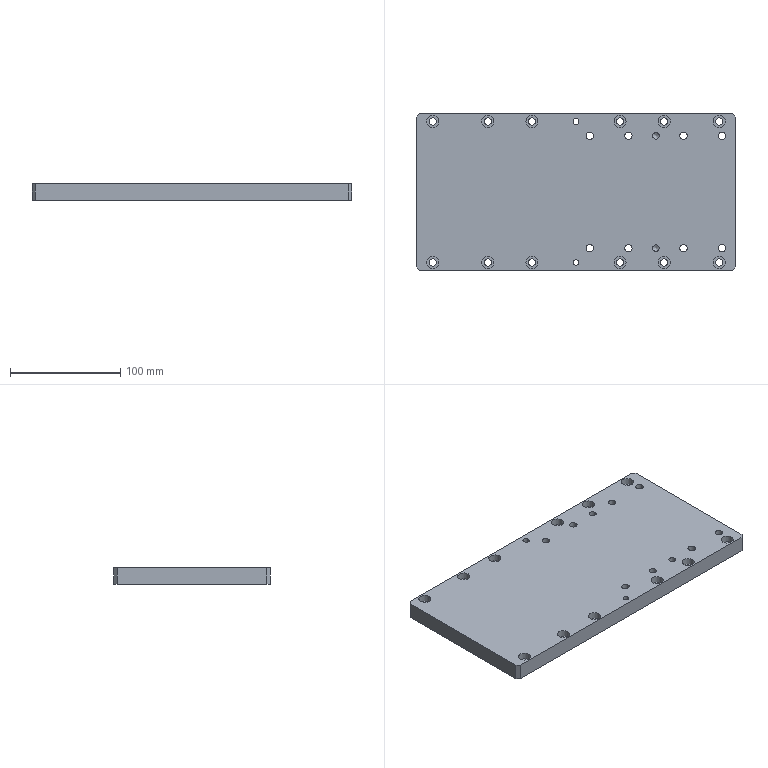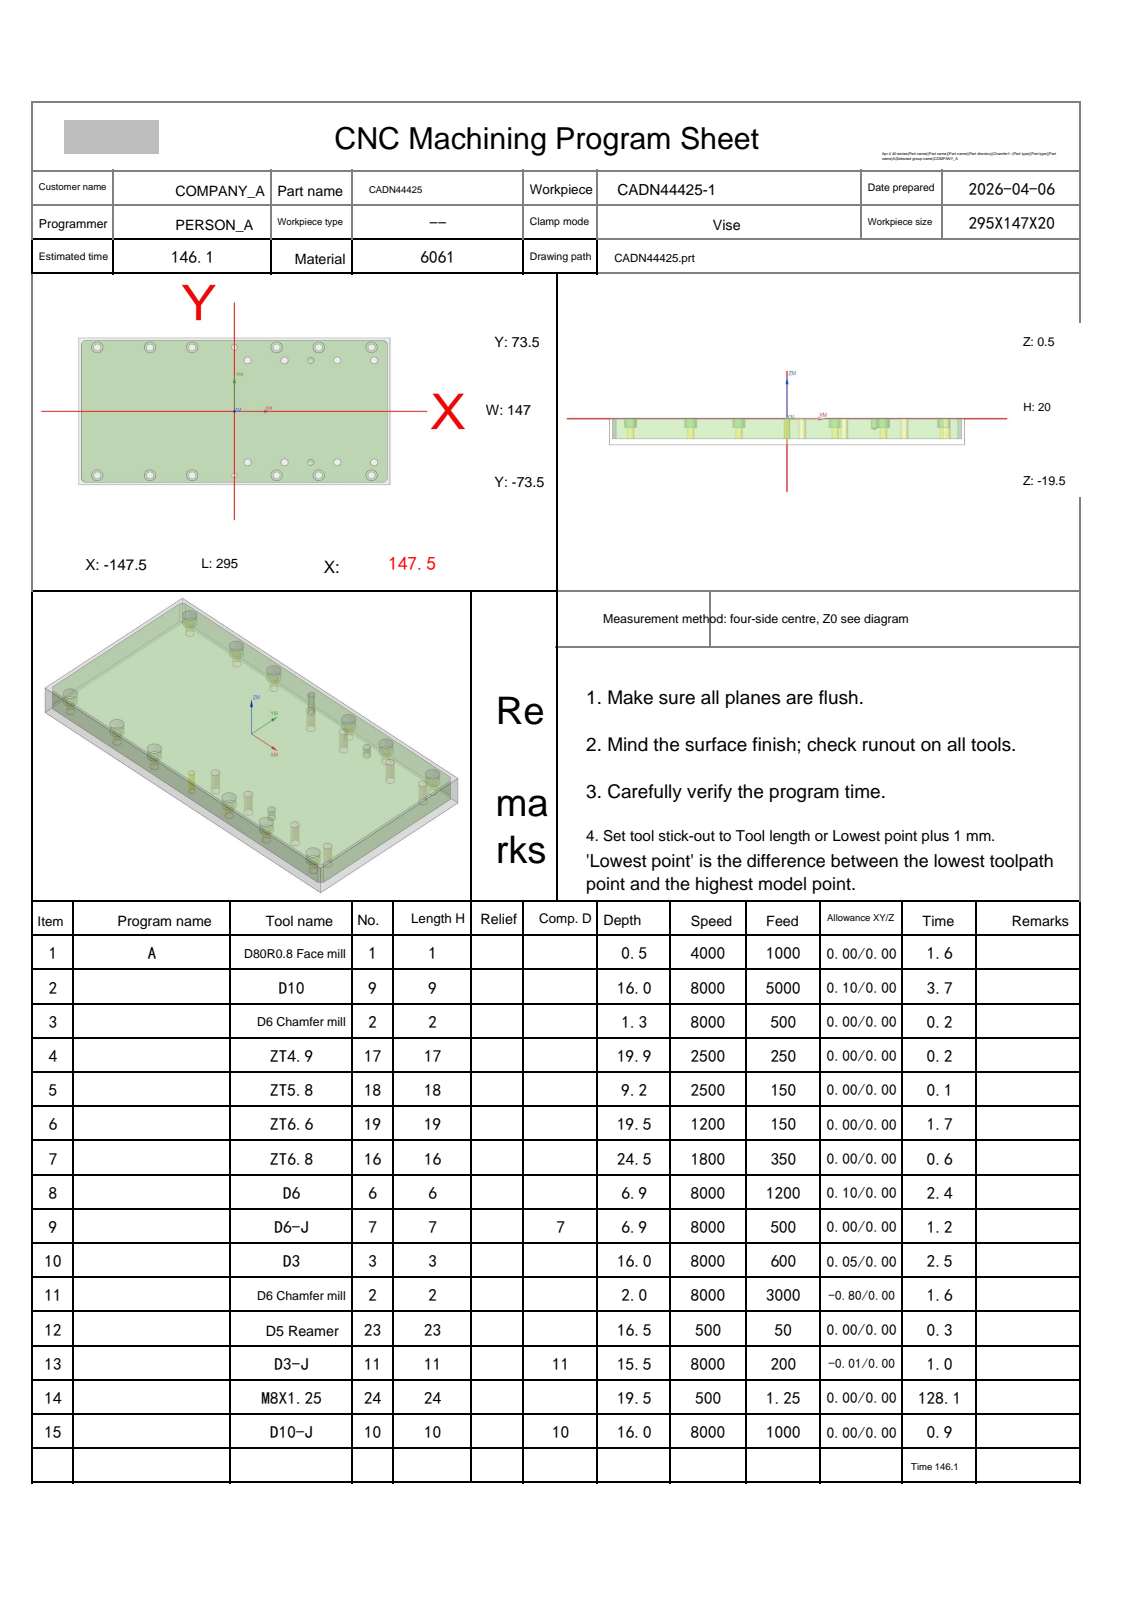NC program | NX | posted by the shop | part box 290 x 142 x 15 mm
Lines 1 to 1801 of 2582, first 1324 of 1799 lines:
%
O0001
(Machine time: 270.74 MIN)
(===Total Tool:14===)
(T1=D80R0.8 Face mill D=80.  R=0.8  D-  H01 Z=0.    )
(T9=D10     D=10.  R=0.   D-  H09 Z=-15.5 )
(T2=D6 Chamfer mill   D=6.   R=0.   D-  H02 Z=-1.5  )
(T17=ZT4.9  D=4.9  DR_a=120 D-  H17 Z=-19.41)
(T18=ZT5.8  D=5.8  DR_a=118 D-  H18 Z=-8.7  )
(T19=ZT6.6  D=6.6  DR_a=118 D-  H19 Z=-18.98)
(T16=ZT6.8  D=6.8  DR_a=118 D-  H16 Z=-24.04)
(T6=D6      D=6.   R=0.   D-  H06 Z=-6.4  )
(T7=D6-J    D=6.   R=0.   D7  H07 Z=-6.4  )
(T3=D3      D=3.   R=0.   D-  H03 Z=-15.5 )
(T23=D5 Reamer   D=5.   DR_a=180 D-  H23 Z=-16.  )
(T11=D3-J   D=3.   R=0.   D11 H11 Z=-15.  )
(T24=M8X1.25 D=6.8  DR_a=180 D-  H24 Z=-19.  )
(T10=D10-J  D=10.  R=0.   D10 H10 Z=-15.5 )
G80 G90 G17 G49 G40
G91 G28 Z0
M01
N1 T01 M06
(D80R0.8 Face mill  D=80. R=0.8 H=01 ce=0.00 di=0.00)
G00 G90 G54 X-190. Y66.6 M03 S4000
G43 H01 Z20.
M08
Z2.
G01 Z0.0 F1000.
X-185.
X185.
Y22.2
X-185.
Y-22.2
X185.
Y-66.6
X-185.
X-190.
Z2.
G00 Z20.
G91 G28 Z0.0
M05
M09
G91 G28 Z0.0
M01
N2 T09 M06
(D10  D=10. R=0. H=09 ce=0.10 di=0.00)
G00 G90 G54 X0.0 Y76.1 M03 S8000
G43 H09 Z20.
M08
Z.5
G01 X142. Z.372 F5000.
G02 X145.606 Y74.606 Z.369 I0.0 J-5.1
G01 X148.606 Y71.606 Z.365
G02 X150.1 Y68. Z.361 I-3.606 J-3.606
G01 Y-68. Z.239
G02 X148.606 Y-71.606 Z.235 I-5.1 J0.0
G01 X145.606 Y-74.606 Z.231
G02 X142. Y-76.1 Z.228 I-3.606 J3.606
G01 X-142. Z-.028
G02 X-145.606 Y-74.606 Z-.031 I0.0 J5.1
G01 X-148.606 Y-71.606 Z-.035
G02 X-150.1 Y-68. Z-.039 I3.606 J3.606
G01 Y68. Z-.161
G02 X-148.606 Y71.606 Z-.165 I5.1 J0.0
G01 X-145.606 Y74.606 Z-.169
G02 X-142. Y76.1 Z-.172 I3.606 J-3.606
G01 X142. Z-.428
G02 X145.606 Y74.606 Z-.431 I0.0 J-5.1
G01 X148.606 Y71.606 Z-.435
G02 X150.1 Y68. Z-.439 I-3.606 J-3.606
G01 Y-68. Z-.561
G02 X148.606 Y-71.606 Z-.565 I-5.1 J0.0
G01 X145.606 Y-74.606 Z-.569
G02 X142. Y-76.1 Z-.572 I-3.606 J3.606
G01 X-142. Z-.828
G02 X-145.606 Y-74.606 Z-.831 I0.0 J5.1
G01 X-148.606 Y-71.606 Z-.835
G02 X-150.1 Y-68. Z-.839 I3.606 J3.606
G01 Y68. Z-.961
G02 X-148.606 Y71.606 Z-.965 I5.1 J0.0
G01 X-145.606 Y74.606 Z-.969
G02 X-142. Y76.1 Z-.972 I3.606 J-3.606
G01 X142. Z-1.228
G02 X145.606 Y74.606 Z-1.231 I0.0 J-5.1
G01 X148.606 Y71.606 Z-1.235
G02 X150.1 Y68. Z-1.239 I-3.606 J-3.606
G01 Y-68. Z-1.361
G02 X148.606 Y-71.606 Z-1.365 I-5.1 J0.0
G01 X145.606 Y-74.606 Z-1.369
G02 X142. Y-76.1 Z-1.372 I-3.606 J3.606
G01 X-142. Z-1.628
G02 X-145.606 Y-74.606 Z-1.631 I0.0 J5.1
G01 X-148.606 Y-71.606 Z-1.635
G02 X-150.1 Y-68. Z-1.639 I3.606 J3.606
G01 Y68. Z-1.761
G02 X-148.606 Y71.606 Z-1.765 I5.1 J0.0
G01 X-145.606 Y74.606 Z-1.769
G02 X-142. Y76.1 Z-1.772 I3.606 J-3.606
G01 X142. Z-2.028
G02 X145.606 Y74.606 Z-2.031 I0.0 J-5.1
G01 X148.606 Y71.606 Z-2.035
G02 X150.1 Y68. Z-2.039 I-3.606 J-3.606
G01 Y-68. Z-2.161
G02 X148.606 Y-71.606 Z-2.165 I-5.1 J0.0
G01 X145.606 Y-74.606 Z-2.169
G02 X142. Y-76.1 Z-2.172 I-3.606 J3.606
G01 X-142. Z-2.428
G02 X-145.606 Y-74.606 Z-2.431 I0.0 J5.1
G01 X-148.606 Y-71.606 Z-2.435
G02 X-150.1 Y-68. Z-2.439 I3.606 J3.606
G01 Y68. Z-2.561
G02 X-148.606 Y71.606 Z-2.565 I5.1 J0.0
G01 X-145.606 Y74.606 Z-2.569
G02 X-142. Y76.1 Z-2.572 I3.606 J-3.606
G01 X142. Z-2.828
G02 X145.606 Y74.606 Z-2.831 I0.0 J-5.1
G01 X148.606 Y71.606 Z-2.835
G02 X150.1 Y68. Z-2.839 I-3.606 J-3.606
G01 Y-68. Z-2.961
G02 X148.606 Y-71.606 Z-2.965 I-5.1 J0.0
G01 X145.606 Y-74.606 Z-2.969
G02 X142. Y-76.1 Z-2.972 I-3.606 J3.606
G01 X-142. Z-3.228
G02 X-145.606 Y-74.606 Z-3.231 I0.0 J5.1
G01 X-148.606 Y-71.606 Z-3.235
G02 X-150.1 Y-68. Z-3.239 I3.606 J3.606
G01 Y68. Z-3.361
G02 X-148.606 Y71.606 Z-3.365 I5.1 J0.0
G01 X-145.606 Y74.606 Z-3.369
G02 X-142. Y76.1 Z-3.372 I3.606 J-3.606
G01 X142. Z-3.628
G02 X145.606 Y74.606 Z-3.631 I0.0 J-5.1
G01 X148.606 Y71.606 Z-3.635
G02 X150.1 Y68. Z-3.639 I-3.606 J-3.606
G01 Y-68. Z-3.761
G02 X148.606 Y-71.606 Z-3.765 I-5.1 J0.0
G01 X145.606 Y-74.606 Z-3.769
G02 X142. Y-76.1 Z-3.772 I-3.606 J3.606
G01 X-142. Z-4.028
G02 X-145.606 Y-74.606 Z-4.031 I0.0 J5.1
G01 X-148.606 Y-71.606 Z-4.035
G02 X-150.1 Y-68. Z-4.039 I3.606 J3.606
G01 Y68. Z-4.161
G02 X-148.606 Y71.606 Z-4.165 I5.1 J0.0
G01 X-145.606 Y74.606 Z-4.169
G02 X-142. Y76.1 Z-4.172 I3.606 J-3.606
G01 X142. Z-4.428
G02 X145.606 Y74.606 Z-4.431 I0.0 J-5.1
G01 X148.606 Y71.606 Z-4.435
G02 X150.1 Y68. Z-4.439 I-3.606 J-3.606
G01 Y-68. Z-4.561
G02 X148.606 Y-71.606 Z-4.565 I-5.1 J0.0
G01 X145.606 Y-74.606 Z-4.569
G02 X142. Y-76.1 Z-4.572 I-3.606 J3.606
G01 X-142. Z-4.828
G02 X-145.606 Y-74.606 Z-4.831 I0.0 J5.1
G01 X-148.606 Y-71.606 Z-4.835
G02 X-150.1 Y-68. Z-4.839 I3.606 J3.606
G01 Y68. Z-4.961
G02 X-148.606 Y71.606 Z-4.965 I5.1 J0.0
G01 X-145.606 Y74.606 Z-4.969
G02 X-142. Y76.1 Z-4.972 I3.606 J-3.606
G01 X142. Z-5.228
G02 X145.606 Y74.606 Z-5.231 I0.0 J-5.1
G01 X148.606 Y71.606 Z-5.235
G02 X150.1 Y68. Z-5.239 I-3.606 J-3.606
G01 Y-68. Z-5.361
G02 X148.606 Y-71.606 Z-5.365 I-5.1 J0.0
G01 X145.606 Y-74.606 Z-5.369
G02 X142. Y-76.1 Z-5.372 I-3.606 J3.606
G01 X-142. Z-5.628
G02 X-145.606 Y-74.606 Z-5.631 I0.0 J5.1
G01 X-148.606 Y-71.606 Z-5.635
G02 X-150.1 Y-68. Z-5.639 I3.606 J3.606
G01 Y68. Z-5.761
G02 X-148.606 Y71.606 Z-5.765 I5.1 J0.0
G01 X-145.606 Y74.606 Z-5.769
G02 X-142. Y76.1 Z-5.772 I3.606 J-3.606
G01 X142. Z-6.028
G02 X145.606 Y74.606 Z-6.031 I0.0 J-5.1
G01 X148.606 Y71.606 Z-6.035
G02 X150.1 Y68. Z-6.039 I-3.606 J-3.606
G01 Y-68. Z-6.161
G02 X148.606 Y-71.606 Z-6.165 I-5.1 J0.0
G01 X145.606 Y-74.606 Z-6.169
G02 X142. Y-76.1 Z-6.172 I-3.606 J3.606
G01 X-142. Z-6.428
G02 X-145.606 Y-74.606 Z-6.431 I0.0 J5.1
G01 X-148.606 Y-71.606 Z-6.435
G02 X-150.1 Y-68. Z-6.439 I3.606 J3.606
G01 Y68. Z-6.561
G02 X-148.606 Y71.606 Z-6.565 I5.1 J0.0
G01 X-145.606 Y74.606 Z-6.569
G02 X-142. Y76.1 Z-6.572 I3.606 J-3.606
G01 X142. Z-6.828
G02 X145.606 Y74.606 Z-6.831 I0.0 J-5.1
G01 X148.606 Y71.606 Z-6.835
G02 X150.1 Y68. Z-6.839 I-3.606 J-3.606
G01 Y-68. Z-6.961
G02 X148.606 Y-71.606 Z-6.965 I-5.1 J0.0
G01 X145.606 Y-74.606 Z-6.969
G02 X142. Y-76.1 Z-6.972 I-3.606 J3.606
G01 X-142. Z-7.228
G02 X-145.606 Y-74.606 Z-7.231 I0.0 J5.1
G01 X-148.606 Y-71.606 Z-7.235
G02 X-150.1 Y-68. Z-7.239 I3.606 J3.606
G01 Y68. Z-7.361
G02 X-148.606 Y71.606 Z-7.365 I5.1 J0.0
G01 X-145.606 Y74.606 Z-7.369
G02 X-142. Y76.1 Z-7.372 I3.606 J-3.606
G01 X142. Z-7.628
G02 X145.606 Y74.606 Z-7.631 I0.0 J-5.1
G01 X148.606 Y71.606 Z-7.635
G02 X150.1 Y68. Z-7.639 I-3.606 J-3.606
G01 Y-68. Z-7.761
G02 X148.606 Y-71.606 Z-7.765 I-5.1 J0.0
G01 X145.606 Y-74.606 Z-7.769
G02 X142. Y-76.1 Z-7.772 I-3.606 J3.606
G01 X-142. Z-8.028
G02 X-145.606 Y-74.606 Z-8.031 I0.0 J5.1
G01 X-148.606 Y-71.606 Z-8.035
G02 X-150.1 Y-68. Z-8.039 I3.606 J3.606
G01 Y68. Z-8.161
G02 X-148.606 Y71.606 Z-8.165 I5.1 J0.0
G01 X-145.606 Y74.606 Z-8.169
G02 X-142. Y76.1 Z-8.172 I3.606 J-3.606
G01 X142. Z-8.428
G02 X145.606 Y74.606 Z-8.431 I0.0 J-5.1
G01 X148.606 Y71.606 Z-8.435
G02 X150.1 Y68. Z-8.439 I-3.606 J-3.606
G01 Y-68. Z-8.561
G02 X148.606 Y-71.606 Z-8.565 I-5.1 J0.0
G01 X145.606 Y-74.606 Z-8.569
G02 X142. Y-76.1 Z-8.572 I-3.606 J3.606
G01 X-142. Z-8.828
G02 X-145.606 Y-74.606 Z-8.831 I0.0 J5.1
G01 X-148.606 Y-71.606 Z-8.835
G02 X-150.1 Y-68. Z-8.839 I3.606 J3.606
G01 Y68. Z-8.961
G02 X-148.606 Y71.606 Z-8.965 I5.1 J0.0
G01 X-145.606 Y74.606 Z-8.969
G02 X-142. Y76.1 Z-8.972 I3.606 J-3.606
G01 X142. Z-9.228
G02 X145.606 Y74.606 Z-9.231 I0.0 J-5.1
G01 X148.606 Y71.606 Z-9.235
G02 X150.1 Y68. Z-9.239 I-3.606 J-3.606
G01 Y-68. Z-9.361
G02 X148.606 Y-71.606 Z-9.365 I-5.1 J0.0
G01 X145.606 Y-74.606 Z-9.369
G02 X142. Y-76.1 Z-9.372 I-3.606 J3.606
G01 X-142. Z-9.628
G02 X-145.606 Y-74.606 Z-9.631 I0.0 J5.1
G01 X-148.606 Y-71.606 Z-9.635
G02 X-150.1 Y-68. Z-9.639 I3.606 J3.606
G01 Y68. Z-9.761
G02 X-148.606 Y71.606 Z-9.765 I5.1 J0.0
G01 X-145.606 Y74.606 Z-9.769
G02 X-142. Y76.1 Z-9.772 I3.606 J-3.606
G01 X142. Z-10.028
G02 X145.606 Y74.606 Z-10.031 I0.0 J-5.1
G01 X148.606 Y71.606 Z-10.035
G02 X150.1 Y68. Z-10.039 I-3.606 J-3.606
G01 Y-68. Z-10.161
G02 X148.606 Y-71.606 Z-10.165 I-5.1 J0.0
G01 X145.606 Y-74.606 Z-10.169
G02 X142. Y-76.1 Z-10.172 I-3.606 J3.606
G01 X-142. Z-10.428
G02 X-145.606 Y-74.606 Z-10.431 I0.0 J5.1
G01 X-148.606 Y-71.606 Z-10.435
G02 X-150.1 Y-68. Z-10.439 I3.606 J3.606
G01 Y68. Z-10.561
G02 X-148.606 Y71.606 Z-10.565 I5.1 J0.0
G01 X-145.606 Y74.606 Z-10.569
G02 X-142. Y76.1 Z-10.572 I3.606 J-3.606
G01 X142. Z-10.828
G02 X145.606 Y74.606 Z-10.831 I0.0 J-5.1
G01 X148.606 Y71.606 Z-10.835
G02 X150.1 Y68. Z-10.839 I-3.606 J-3.606
G01 Y-68. Z-10.961
G02 X148.606 Y-71.606 Z-10.965 I-5.1 J0.0
G01 X145.606 Y-74.606 Z-10.969
G02 X142. Y-76.1 Z-10.972 I-3.606 J3.606
G01 X-142. Z-11.228
G02 X-145.606 Y-74.606 Z-11.231 I0.0 J5.1
G01 X-148.606 Y-71.606 Z-11.235
G02 X-150.1 Y-68. Z-11.239 I3.606 J3.606
G01 Y68. Z-11.361
G02 X-148.606 Y71.606 Z-11.365 I5.1 J0.0
G01 X-145.606 Y74.606 Z-11.369
G02 X-142. Y76.1 Z-11.372 I3.606 J-3.606
G01 X142. Z-11.628
G02 X145.606 Y74.606 Z-11.631 I0.0 J-5.1
G01 X148.606 Y71.606 Z-11.635
G02 X150.1 Y68. Z-11.639 I-3.606 J-3.606
G01 Y-68. Z-11.761
G02 X148.606 Y-71.606 Z-11.765 I-5.1 J0.0
G01 X145.606 Y-74.606 Z-11.769
G02 X142. Y-76.1 Z-11.772 I-3.606 J3.606
G01 X-142. Z-12.028
G02 X-145.606 Y-74.606 Z-12.031 I0.0 J5.1
G01 X-148.606 Y-71.606 Z-12.035
G02 X-150.1 Y-68. Z-12.039 I3.606 J3.606
G01 Y68. Z-12.161
G02 X-148.606 Y71.606 Z-12.165 I5.1 J0.0
G01 X-145.606 Y74.606 Z-12.169
G02 X-142. Y76.1 Z-12.172 I3.606 J-3.606
G01 X142. Z-12.428
G02 X145.606 Y74.606 Z-12.431 I0.0 J-5.1
G01 X148.606 Y71.606 Z-12.435
G02 X150.1 Y68. Z-12.439 I-3.606 J-3.606
G01 Y-68. Z-12.561
G02 X148.606 Y-71.606 Z-12.565 I-5.1 J0.0
G01 X145.606 Y-74.606 Z-12.569
G02 X142. Y-76.1 Z-12.572 I-3.606 J3.606
G01 X-142. Z-12.828
G02 X-145.606 Y-74.606 Z-12.831 I0.0 J5.1
G01 X-148.606 Y-71.606 Z-12.835
G02 X-150.1 Y-68. Z-12.839 I3.606 J3.606
G01 Y68. Z-12.961
G02 X-148.606 Y71.606 Z-12.965 I5.1 J0.0
G01 X-145.606 Y74.606 Z-12.969
G02 X-142. Y76.1 Z-12.972 I3.606 J-3.606
G01 X142. Z-13.228
G02 X145.606 Y74.606 Z-13.231 I0.0 J-5.1
G01 X148.606 Y71.606 Z-13.235
G02 X150.1 Y68. Z-13.239 I-3.606 J-3.606
G01 Y-68. Z-13.361
G02 X148.606 Y-71.606 Z-13.365 I-5.1 J0.0
G01 X145.606 Y-74.606 Z-13.369
G02 X142. Y-76.1 Z-13.372 I-3.606 J3.606
G01 X-142. Z-13.628
G02 X-145.606 Y-74.606 Z-13.631 I0.0 J5.1
G01 X-148.606 Y-71.606 Z-13.635
G02 X-150.1 Y-68. Z-13.639 I3.606 J3.606
G01 Y68. Z-13.761
G02 X-148.606 Y71.606 Z-13.765 I5.1 J0.0
G01 X-145.606 Y74.606 Z-13.769
G02 X-142. Y76.1 Z-13.772 I3.606 J-3.606
G01 X142. Z-14.028
G02 X145.606 Y74.606 Z-14.031 I0.0 J-5.1
G01 X148.606 Y71.606 Z-14.035
G02 X150.1 Y68. Z-14.039 I-3.606 J-3.606
G01 Y-68. Z-14.161
G02 X148.606 Y-71.606 Z-14.165 I-5.1 J0.0
G01 X145.606 Y-74.606 Z-14.169
G02 X142. Y-76.1 Z-14.172 I-3.606 J3.606
G01 X-142. Z-14.428
G02 X-145.606 Y-74.606 Z-14.431 I0.0 J5.1
G01 X-148.606 Y-71.606 Z-14.435
G02 X-150.1 Y-68. Z-14.439 I3.606 J3.606
G01 Y68. Z-14.561
G02 X-148.606 Y71.606 Z-14.565 I5.1 J0.0
G01 X-145.606 Y74.606 Z-14.569
G02 X-142. Y76.1 Z-14.572 I3.606 J-3.606
G01 X142. Z-14.828
G02 X145.606 Y74.606 Z-14.831 I0.0 J-5.1
G01 X148.606 Y71.606 Z-14.835
G02 X150.1 Y68. Z-14.839 I-3.606 J-3.606
G01 Y-68. Z-14.961
G02 X148.606 Y-71.606 Z-14.965 I-5.1 J0.0
G01 X145.606 Y-74.606 Z-14.969
G02 X142. Y-76.1 Z-14.972 I-3.606 J3.606
G01 X-142. Z-15.228
G02 X-145.606 Y-74.606 Z-15.231 I0.0 J5.1
G01 X-148.606 Y-71.606 Z-15.235
G02 X-150.1 Y-68. Z-15.239 I3.606 J3.606
G01 Y68. Z-15.361
G02 X-148.606 Y71.606 Z-15.365 I5.1 J0.0
G01 X-145.606 Y74.606 Z-15.369
G02 X-142. Y76.1 Z-15.372 I3.606 J-3.606
G01 X0.0 Z-15.5
X142.
G02 X145.606 Y74.606 I0.0 J-5.1
G01 X148.606 Y71.606
G02 X150.1 Y68. I-3.606 J-3.606
G01 Y-68.
G02 X148.606 Y-71.606 I-5.1 J0.0
G01 X145.606 Y-74.606
G02 X142. Y-76.1 I-3.606 J3.606
G01 X-142.
G02 X-145.606 Y-74.606 I0.0 J5.1
G01 X-148.606 Y-71.606
G02 X-150.1 Y-68. I3.606 J3.606
G01 Y68.
G02 X-148.606 Y71.606 I5.1 J0.0
G01 X-145.606 Y74.606
G02 X-142. Y76.1 I3.606 J-3.606
G01 X0.0
X.5
Z-14.5
G00 Z20.
G91 G28 Z0.0
M05
M09
G91 G28 Z0.0
M01
N3 T02 M06
(D6 Chamfer mill  D=6. R=0. H=02 ce=0.00 di=0.00)
G00 G90 G54 X-130. Y64. M03 S8000
G43 H02 Z20.
M08
G98 G81 X-130. Y64. Z-.8 R1. F500.
X-80.
X-40.
X12.5 Y51.
X40. Y64.
X47.5 Y51.
X72.5
X80. Y64.
X97.5 Y51.
X130. Y64.
X132.5 Y51.
Y-51.
X130. Y-64.
X97.5 Y-51.
X80. Y-64.
X72.5 Y-51.
X47.5
X40. Y-64.
X12.5 Y-51.
X0.0 Y-64.
X-40.
X-80.
X-130.
X0.0 Y63.5
G80
G00 Z20.
G91 G28 Z0.0
M05
M09
G91 G28 Z0.0
M01
N4 T17 M06
(ZT4.9 D=4.9 DR_a=120 H=17)
G00 G90 G54 X0.0 Y-64. M03 S2500
G43 H17 Z20.
M08
G98 G83 X0.0 Y-64. Z-19.415 R1. F250. Q2.
Y63.5
G80
G00 Z20.
G91 G28 Z0.0
M05
M09
G91 G28 Z0.0
M01
N5 T18 M06
(ZT5.8 D=5.8 DR_a=118 H=18)
G00 G90 G54 X72.5 Y51. M03 S2500
G43 H18 Z20.
M08
G98 G83 X72.5 Y51. Z-8.703 R1. F150. Q2.
Y-51.
G80
G00 Z20.
G91 G28 Z0.0
M05
M09
G91 G28 Z0.0
M01
N6 T19 M06
(ZT6.6 D=6.6 DR_a=118 H=19)
G00 G90 G54 X130. Y64. M03 S1200
G43 H19 Z20.
M08
G98 G83 X130. Y64. Z-18.983 R1. F150. Q2.
X80.
X40.
X-40.
X-80.
X-130.
Y-64.
X-80.
X-40.
X40.
X80.
X130.
G80
G00 Z20.
G91 G28 Z0.0
M05
M09
G91 G28 Z0.0
M01
N7 T16 M06
(ZT6.8 D=6.8 DR_a=118 H=16)
G00 G90 G54 X132.5 Y-51. M03 S1800
G43 H16 Z20.
M08
G98 G83 X132.5 Y-51. Z-24.043 R1. F350. Q3.
X97.5
X47.5
X12.5
Y51.
X47.5
X97.5
X132.5
G80
G00 Z20.
G91 G28 Z0.0
M05
M09
G91 G28 Z0.0
M01
N8 T06 M06
(D6  D=6. R=0. H=06 ce=0.10 di=0.00)
G00 G90 G54 X130. Y-64. M03 S8000
G43 H06 Z20.
M08
Z.5
G03 X131.2 Y-65.2 I1.2 J0.0 F1200.
X132.4 Y-64. I0.0 J1.2
X132.4 Y-64. Z0.0 I-2.4 J0.0
X132.4 Y-64. Z-.5 I-2.4 J0.0
X132.4 Y-64. Z-1. I-2.4 J0.0
X132.4 Y-64. Z-1.5 I-2.4 J0.0
X132.4 Y-64. Z-2. I-2.4 J0.0
X132.4 Y-64. Z-2.5 I-2.4 J0.0
X132.4 Y-64. Z-3. I-2.4 J0.0
X132.4 Y-64. Z-3.5 I-2.4 J0.0
X132.4 Y-64. Z-4. I-2.4 J0.0
X132.4 Y-64. Z-4.5 I-2.4 J0.0
X132.4 Y-64. Z-5. I-2.4 J0.0
X132.4 Y-64. Z-5.5 I-2.4 J0.0
X132.4 Y-64. Z-6. I-2.4 J0.0
X130.742 Y-66.283 Z-6.4 I-2.4 J0.0
X132.4 Y-64. I-.742 J2.283
X130. Y-61.6 I-2.4 J0.0
X127.6 Y-64. I0.0 J-2.4
X130. Y-66.4 I2.4 J0.0
X130.742 Y-66.283 I0.0 J2.4
X131.571 Y-65.141 I-.371 J1.141
X130.371 Y-63.941 I-1.2 J0.0
X130. Y-64. I0.0 J-1.2
G00 Z20.
X80.
Z.5
G03 X81.2 Y-65.2 I1.2 J0.0
X82.4 Y-64. I0.0 J1.2
X82.4 Y-64. Z0.0 I-2.4 J0.0
X82.4 Y-64. Z-.5 I-2.4 J0.0
X82.4 Y-64. Z-1. I-2.4 J0.0
X82.4 Y-64. Z-1.5 I-2.4 J0.0
X82.4 Y-64. Z-2. I-2.4 J0.0
X82.4 Y-64. Z-2.5 I-2.4 J0.0
X82.4 Y-64. Z-3. I-2.4 J0.0
X82.4 Y-64. Z-3.5 I-2.4 J0.0
X82.4 Y-64. Z-4. I-2.4 J0.0
X82.4 Y-64. Z-4.5 I-2.4 J0.0
X82.4 Y-64. Z-5. I-2.4 J0.0
X82.4 Y-64. Z-5.5 I-2.4 J0.0
X82.4 Y-64. Z-6. I-2.4 J0.0
X80.742 Y-66.283 Z-6.4 I-2.4 J0.0
X82.4 Y-64. I-.742 J2.283
X80. Y-61.6 I-2.4 J0.0
X77.6 Y-64. I0.0 J-2.4
X80. Y-66.4 I2.4 J0.0
X80.742 Y-66.283 I0.0 J2.4
X81.571 Y-65.141 I-.371 J1.141
X80.371 Y-63.941 I-1.2 J0.0
X80. Y-64. I0.0 J-1.2
G00 Z20.
X40.
Z.5
G03 X41.2 Y-65.2 I1.2 J0.0
X42.4 Y-64. I0.0 J1.2
X42.4 Y-64. Z0.0 I-2.4 J0.0
X42.4 Y-64. Z-.5 I-2.4 J0.0
X42.4 Y-64. Z-1. I-2.4 J0.0
X42.4 Y-64. Z-1.5 I-2.4 J0.0
X42.4 Y-64. Z-2. I-2.4 J0.0
X42.4 Y-64. Z-2.5 I-2.4 J0.0
X42.4 Y-64. Z-3. I-2.4 J0.0
X42.4 Y-64. Z-3.5 I-2.4 J0.0
X42.4 Y-64. Z-4. I-2.4 J0.0
X42.4 Y-64. Z-4.5 I-2.4 J0.0
X42.4 Y-64. Z-5. I-2.4 J0.0
X42.4 Y-64. Z-5.5 I-2.4 J0.0
X42.4 Y-64. Z-6. I-2.4 J0.0
X40.742 Y-66.283 Z-6.4 I-2.4 J0.0
X42.4 Y-64. I-.742 J2.283
X40. Y-61.6 I-2.4 J0.0
X37.6 Y-64. I0.0 J-2.4
X40. Y-66.4 I2.4 J0.0
X40.742 Y-66.283 I0.0 J2.4
X41.571 Y-65.141 I-.371 J1.141
X40.371 Y-63.941 I-1.2 J0.0
X40. Y-64. I0.0 J-1.2
G00 Z20.
X-40.
Z.5
G03 X-38.8 Y-65.2 I1.2 J0.0
X-37.6 Y-64. I0.0 J1.2
X-37.6 Y-64. Z0.0 I-2.4 J0.0
X-37.6 Y-64. Z-.5 I-2.4 J0.0
X-37.6 Y-64. Z-1. I-2.4 J0.0
X-37.6 Y-64. Z-1.5 I-2.4 J0.0
X-37.6 Y-64. Z-2. I-2.4 J0.0
X-37.6 Y-64. Z-2.5 I-2.4 J0.0
X-37.6 Y-64. Z-3. I-2.4 J0.0
X-37.6 Y-64. Z-3.5 I-2.4 J0.0
X-37.6 Y-64. Z-4. I-2.4 J0.0
X-37.6 Y-64. Z-4.5 I-2.4 J0.0
X-37.6 Y-64. Z-5. I-2.4 J0.0
X-37.6 Y-64. Z-5.5 I-2.4 J0.0
X-37.6 Y-64. Z-6. I-2.4 J0.0
X-39.258 Y-66.283 Z-6.4 I-2.4 J0.0
X-37.6 Y-64. I-.742 J2.283
X-40. Y-61.6 I-2.4 J0.0
X-42.4 Y-64. I0.0 J-2.4
X-40. Y-66.4 I2.4 J0.0
X-39.258 Y-66.283 I0.0 J2.4
X-38.429 Y-65.141 I-.371 J1.141
X-39.629 Y-63.941 I-1.2 J0.0
X-40. Y-64. I0.0 J-1.2
G00 Z20.
X-80.
Z.5
G03 X-78.8 Y-65.2 I1.2 J0.0
X-77.6 Y-64. I0.0 J1.2
X-77.6 Y-64. Z0.0 I-2.4 J0.0
X-77.6 Y-64. Z-.5 I-2.4 J0.0
X-77.6 Y-64. Z-1. I-2.4 J0.0
X-77.6 Y-64. Z-1.5 I-2.4 J0.0
X-77.6 Y-64. Z-2. I-2.4 J0.0
X-77.6 Y-64. Z-2.5 I-2.4 J0.0
X-77.6 Y-64. Z-3. I-2.4 J0.0
X-77.6 Y-64. Z-3.5 I-2.4 J0.0
X-77.6 Y-64. Z-4. I-2.4 J0.0
X-77.6 Y-64. Z-4.5 I-2.4 J0.0
X-77.6 Y-64. Z-5. I-2.4 J0.0
X-77.6 Y-64. Z-5.5 I-2.4 J0.0
X-77.6 Y-64. Z-6. I-2.4 J0.0
X-79.258 Y-66.283 Z-6.4 I-2.4 J0.0
X-77.6 Y-64. I-.742 J2.283
X-80. Y-61.6 I-2.4 J0.0
X-82.4 Y-64. I0.0 J-2.4
X-80. Y-66.4 I2.4 J0.0
X-79.258 Y-66.283 I0.0 J2.4
X-78.429 Y-65.141 I-.371 J1.141
X-79.629 Y-63.941 I-1.2 J0.0
X-80. Y-64. I0.0 J-1.2
G00 Z20.
X-130.
Z.5
G03 X-128.8 Y-65.2 I1.2 J0.0
X-127.6 Y-64. I0.0 J1.2
X-127.6 Y-64. Z0.0 I-2.4 J0.0
X-127.6 Y-64. Z-.5 I-2.4 J0.0
X-127.6 Y-64. Z-1. I-2.4 J0.0
X-127.6 Y-64. Z-1.5 I-2.4 J0.0
X-127.6 Y-64. Z-2. I-2.4 J0.0
X-127.6 Y-64. Z-2.5 I-2.4 J0.0
X-127.6 Y-64. Z-3. I-2.4 J0.0
X-127.6 Y-64. Z-3.5 I-2.4 J0.0
X-127.6 Y-64. Z-4. I-2.4 J0.0
X-127.6 Y-64. Z-4.5 I-2.4 J0.0
X-127.6 Y-64. Z-5. I-2.4 J0.0
X-127.6 Y-64. Z-5.5 I-2.4 J0.0
X-127.6 Y-64. Z-6. I-2.4 J0.0
X-129.258 Y-66.283 Z-6.4 I-2.4 J0.0
X-127.6 Y-64. I-.742 J2.283
X-130. Y-61.6 I-2.4 J0.0
X-132.4 Y-64. I0.0 J-2.4
X-130. Y-66.4 I2.4 J0.0
X-129.258 Y-66.283 I0.0 J2.4
X-128.429 Y-65.141 I-.371 J1.141
X-129.629 Y-63.941 I-1.2 J0.0
X-130. Y-64. I0.0 J-1.2
G00 Z20.
Y64.
Z.5
G03 X-128.8 Y62.8 I1.2 J0.0
X-127.6 Y64. I0.0 J1.2
X-127.6 Y64. Z0.0 I-2.4 J0.0
X-127.6 Y64. Z-.5 I-2.4 J0.0
X-127.6 Y64. Z-1. I-2.4 J0.0
X-127.6 Y64. Z-1.5 I-2.4 J0.0
X-127.6 Y64. Z-2. I-2.4 J0.0
X-127.6 Y64. Z-2.5 I-2.4 J0.0
X-127.6 Y64. Z-3. I-2.4 J0.0
X-127.6 Y64. Z-3.5 I-2.4 J0.0
X-127.6 Y64. Z-4. I-2.4 J0.0
X-127.6 Y64. Z-4.5 I-2.4 J0.0
X-127.6 Y64. Z-5. I-2.4 J0.0
X-127.6 Y64. Z-5.5 I-2.4 J0.0
X-127.6 Y64. Z-6. I-2.4 J0.0
X-129.258 Y61.717 Z-6.4 I-2.4 J0.0
X-127.6 Y64. I-.742 J2.283
X-130. Y66.4 I-2.4 J0.0
X-132.4 Y64. I0.0 J-2.4
X-130. Y61.6 I2.4 J0.0
X-129.258 Y61.717 I0.0 J2.4
X-128.429 Y62.859 I-.371 J1.141
X-129.629 Y64.059 I-1.2 J0.0
X-130. Y64. I0.0 J-1.2
G00 Z20.
X-80.
Z.5
G03 X-78.8 Y62.8 I1.2 J0.0
X-77.6 Y64. I0.0 J1.2
X-77.6 Y64. Z0.0 I-2.4 J0.0
X-77.6 Y64. Z-.5 I-2.4 J0.0
X-77.6 Y64. Z-1. I-2.4 J0.0
X-77.6 Y64. Z-1.5 I-2.4 J0.0
X-77.6 Y64. Z-2. I-2.4 J0.0
X-77.6 Y64. Z-2.5 I-2.4 J0.0
X-77.6 Y64. Z-3. I-2.4 J0.0
X-77.6 Y64. Z-3.5 I-2.4 J0.0
X-77.6 Y64. Z-4. I-2.4 J0.0
X-77.6 Y64. Z-4.5 I-2.4 J0.0
X-77.6 Y64. Z-5. I-2.4 J0.0
X-77.6 Y64. Z-5.5 I-2.4 J0.0
X-77.6 Y64. Z-6. I-2.4 J0.0
X-79.258 Y61.717 Z-6.4 I-2.4 J0.0
X-77.6 Y64. I-.742 J2.283
X-80. Y66.4 I-2.4 J0.0
X-82.4 Y64. I0.0 J-2.4
X-80. Y61.6 I2.4 J0.0
X-79.258 Y61.717 I0.0 J2.4
X-78.429 Y62.859 I-.371 J1.141
X-79.629 Y64.059 I-1.2 J0.0
X-80. Y64. I0.0 J-1.2
G00 Z20.
X-40.
Z.5
G03 X-38.8 Y62.8 I1.2 J0.0
X-37.6 Y64. I0.0 J1.2
X-37.6 Y64. Z0.0 I-2.4 J0.0
X-37.6 Y64. Z-.5 I-2.4 J0.0
X-37.6 Y64. Z-1. I-2.4 J0.0
X-37.6 Y64. Z-1.5 I-2.4 J0.0
X-37.6 Y64. Z-2. I-2.4 J0.0
X-37.6 Y64. Z-2.5 I-2.4 J0.0
X-37.6 Y64. Z-3. I-2.4 J0.0
X-37.6 Y64. Z-3.5 I-2.4 J0.0
X-37.6 Y64. Z-4. I-2.4 J0.0
X-37.6 Y64. Z-4.5 I-2.4 J0.0
X-37.6 Y64. Z-5. I-2.4 J0.0
X-37.6 Y64. Z-5.5 I-2.4 J0.0
X-37.6 Y64. Z-6. I-2.4 J0.0
X-39.258 Y61.717 Z-6.4 I-2.4 J0.0
X-37.6 Y64. I-.742 J2.283
X-40. Y66.4 I-2.4 J0.0
X-42.4 Y64. I0.0 J-2.4
X-40. Y61.6 I2.4 J0.0
X-39.258 Y61.717 I0.0 J2.4
X-38.429 Y62.859 I-.371 J1.141
X-39.629 Y64.059 I-1.2 J0.0
X-40. Y64. I0.0 J-1.2
G00 Z20.
X40.
Z.5
G03 X41.2 Y62.8 I1.2 J0.0
X42.4 Y64. I0.0 J1.2
X42.4 Y64. Z0.0 I-2.4 J0.0
X42.4 Y64. Z-.5 I-2.4 J0.0
X42.4 Y64. Z-1. I-2.4 J0.0
X42.4 Y64. Z-1.5 I-2.4 J0.0
X42.4 Y64. Z-2. I-2.4 J0.0
X42.4 Y64. Z-2.5 I-2.4 J0.0
X42.4 Y64. Z-3. I-2.4 J0.0
X42.4 Y64. Z-3.5 I-2.4 J0.0
X42.4 Y64. Z-4. I-2.4 J0.0
X42.4 Y64. Z-4.5 I-2.4 J0.0
X42.4 Y64. Z-5. I-2.4 J0.0
X42.4 Y64. Z-5.5 I-2.4 J0.0
X42.4 Y64. Z-6. I-2.4 J0.0
X40.742 Y61.717 Z-6.4 I-2.4 J0.0
X42.4 Y64. I-.742 J2.283
X40. Y66.4 I-2.4 J0.0
X37.6 Y64. I0.0 J-2.4
X40. Y61.6 I2.4 J0.0
X40.742 Y61.717 I0.0 J2.4
X41.571 Y62.859 I-.371 J1.141
X40.371 Y64.059 I-1.2 J0.0
X40. Y64. I0.0 J-1.2
G00 Z20.
X80.
Z.5
G03 X81.2 Y62.8 I1.2 J0.0
X82.4 Y64. I0.0 J1.2
X82.4 Y64. Z0.0 I-2.4 J0.0
X82.4 Y64. Z-.5 I-2.4 J0.0
X82.4 Y64. Z-1. I-2.4 J0.0
X82.4 Y64. Z-1.5 I-2.4 J0.0
X82.4 Y64. Z-2. I-2.4 J0.0
X82.4 Y64. Z-2.5 I-2.4 J0.0
X82.4 Y64. Z-3. I-2.4 J0.0
X82.4 Y64. Z-3.5 I-2.4 J0.0
X82.4 Y64. Z-4. I-2.4 J0.0
X82.4 Y64. Z-4.5 I-2.4 J0.0
X82.4 Y64. Z-5. I-2.4 J0.0
X82.4 Y64. Z-5.5 I-2.4 J0.0
X82.4 Y64. Z-6. I-2.4 J0.0
X80.742 Y61.717 Z-6.4 I-2.4 J0.0
X82.4 Y64. I-.742 J2.283
X80. Y66.4 I-2.4 J0.0
X77.6 Y64. I0.0 J-2.4
X80. Y61.6 I2.4 J0.0
X80.742 Y61.717 I0.0 J2.4
X81.571 Y62.859 I-.371 J1.141
X80.371 Y64.059 I-1.2 J0.0
X80. Y64. I0.0 J-1.2
G00 Z20.
X130.
Z.5
G03 X131.2 Y62.8 I1.2 J0.0
X132.4 Y64. I0.0 J1.2
X132.4 Y64. Z0.0 I-2.4 J0.0
X132.4 Y64. Z-.5 I-2.4 J0.0
X132.4 Y64. Z-1. I-2.4 J0.0
X132.4 Y64. Z-1.5 I-2.4 J0.0
X132.4 Y64. Z-2. I-2.4 J0.0
X132.4 Y64. Z-2.5 I-2.4 J0.0
X132.4 Y64. Z-3. I-2.4 J0.0
X132.4 Y64. Z-3.5 I-2.4 J0.0
X132.4 Y64. Z-4. I-2.4 J0.0
X132.4 Y64. Z-4.5 I-2.4 J0.0
X132.4 Y64. Z-5. I-2.4 J0.0
X132.4 Y64. Z-5.5 I-2.4 J0.0
X132.4 Y64. Z-6. I-2.4 J0.0
X130.742 Y61.717 Z-6.4 I-2.4 J0.0
X132.4 Y64. I-.742 J2.283
X130. Y66.4 I-2.4 J0.0
X127.6 Y64. I0.0 J-2.4
X130. Y61.6 I2.4 J0.0
X130.742 Y61.717 I0.0 J2.4
X131.571 Y62.859 I-.371 J1.141
X130.371 Y64.059 I-1.2 J0.0
X130. Y64. I0.0 J-1.2
G00 Z20.
G91 G28 Z0.0
M05
M09
G91 G28 Z0.0
M01
N9 T07 M06
(D6-J  D=6. R=0. H=07 ce=0.00 di=0.00)
G00 G90 G54 X130. Y-64. M03 S8000
G43 H07 Z20.
M08
Z0.0
G41 D07
G01 X130.032 Y-64.197 F500.
G03 X131.258 Y-65.242 I1.226 J.197
X132.5 Y-64. I0.0 J1.242
X132.5 Y-64. Z-5. I-2.5 J0.0
X129.532 Y-61.544 Z-6.4 I-2.5 J0.0
X127.5 Y-64. I.468 J-2.456
X130. Y-66.5 I2.5 J0.0
X132.5 Y-64. I0.0 J2.5
X130. Y-61.5 I-2.5 J0.0
X129.532 Y-61.544 I0.0 J-2.5
X128.522 Y-62.764 I.233 J-1.22
X129.764 Y-64.006 I1.242 J0.0
G01 X129.8
G40 X130. Y-64.
G00 Z20.
X80.
Z0.0
G41 D07
G01 X80.032 Y-64.197
G03 X81.258 Y-65.242 I1.226 J.197
X82.5 Y-64. I0.0 J1.242
X82.5 Y-64. Z-5. I-2.5 J0.0
X79.532 Y-61.544 Z-6.4 I-2.5 J0.0
X77.5 Y-64. I.468 J-2.456
X80. Y-66.5 I2.5 J0.0
X82.5 Y-64. I0.0 J2.5
X80. Y-61.5 I-2.5 J0.0
X79.532 Y-61.544 I0.0 J-2.5
X78.522 Y-62.764 I.233 J-1.22
X79.764 Y-64.006 I1.242 J0.0
G01 X79.8
G40 X80. Y-64.
G00 Z20.
X40.
Z0.0
G41 D07
G01 X40.032 Y-64.197
G03 X41.258 Y-65.242 I1.226 J.197
X42.5 Y-64. I0.0 J1.242
X42.5 Y-64. Z-5. I-2.5 J0.0
X39.532 Y-61.544 Z-6.4 I-2.5 J0.0
X37.5 Y-64. I.468 J-2.456
X40. Y-66.5 I2.5 J0.0
X42.5 Y-64. I0.0 J2.5
X40. Y-61.5 I-2.5 J0.0
X39.532 Y-61.544 I0.0 J-2.5
X38.522 Y-62.764 I.233 J-1.22
X39.764 Y-64.006 I1.242 J0.0
G01 X39.8
G40 X40. Y-64.
G00 Z20.
X-40.
Z0.0
G41 D07
G01 X-39.968 Y-64.197
G03 X-38.742 Y-65.242 I1.226 J.197
X-37.5 Y-64. I0.0 J1.242
X-37.5 Y-64. Z-5. I-2.5 J0.0
X-40.468 Y-61.544 Z-6.4 I-2.5 J0.0
X-42.5 Y-64. I.468 J-2.456
X-40. Y-66.5 I2.5 J0.0
X-37.5 Y-64. I0.0 J2.5
X-40. Y-61.5 I-2.5 J0.0
X-40.468 Y-61.544 I0.0 J-2.5
X-41.478 Y-62.764 I.233 J-1.22
X-40.236 Y-64.006 I1.242 J0.0
G01 X-40.2
G40 X-40. Y-64.
G00 Z20.
X-80.
Z0.0
G41 D07
G01 X-79.968 Y-64.197
G03 X-78.742 Y-65.242 I1.226 J.197
X-77.5 Y-64. I0.0 J1.242
X-77.5 Y-64. Z-5. I-2.5 J0.0
X-80.468 Y-61.544 Z-6.4 I-2.5 J0.0
X-82.5 Y-64. I.468 J-2.456
X-80. Y-66.5 I2.5 J0.0
X-77.5 Y-64. I0.0 J2.5
X-80. Y-61.5 I-2.5 J0.0
X-80.468 Y-61.544 I0.0 J-2.5
X-81.478 Y-62.764 I.233 J-1.22
X-80.236 Y-64.006 I1.242 J0.0
G01 X-80.2
G40 X-80. Y-64.
G00 Z20.
X-130.
Z0.0
G41 D07
G01 X-129.968 Y-64.197
G03 X-128.742 Y-65.242 I1.226 J.197
X-127.5 Y-64. I0.0 J1.242
X-127.5 Y-64. Z-5. I-2.5 J0.0
X-130.468 Y-61.544 Z-6.4 I-2.5 J0.0
X-132.5 Y-64. I.468 J-2.456
X-130. Y-66.5 I2.5 J0.0
X-127.5 Y-64. I0.0 J2.5
X-130. Y-61.5 I-2.5 J0.0
X-130.468 Y-61.544 I0.0 J-2.5
X-131.478 Y-62.764 I.233 J-1.22
X-130.236 Y-64.006 I1.242 J0.0
G01 X-130.2
G40 X-130. Y-64.
G00 Z20.
Y64.
Z0.0
G41 D07
G01 X-129.968 Y63.803
G03 X-128.742 Y62.758 I1.226 J.197
X-127.5 Y64. I0.0 J1.242
X-127.5 Y64. Z-5. I-2.5 J0.0
X-130.468 Y66.456 Z-6.4 I-2.5 J0.0
X-132.5 Y64. I.468 J-2.456
X-130. Y61.5 I2.5 J0.0
X-127.5 Y64. I0.0 J2.5
X-130. Y66.5 I-2.5 J0.0
X-130.468 Y66.456 I0.0 J-2.5
X-131.478 Y65.236 I.233 J-1.22
X-130.236 Y63.994 I1.242 J0.0
G01 X-130.2
G40 X-130. Y64.
G00 Z20.
X-80.
Z0.0
G41 D07
G01 X-79.968 Y63.803
G03 X-78.742 Y62.758 I1.226 J.197
X-77.5 Y64. I0.0 J1.242
X-77.5 Y64. Z-5. I-2.5 J0.0
X-80.468 Y66.456 Z-6.4 I-2.5 J0.0
X-82.5 Y64. I.468 J-2.456
X-80. Y61.5 I2.5 J0.0
X-77.5 Y64. I0.0 J2.5
X-80. Y66.5 I-2.5 J0.0
X-80.468 Y66.456 I0.0 J-2.5
X-81.478 Y65.236 I.233 J-1.22
X-80.236 Y63.994 I1.242 J0.0
G01 X-80.2
G40 X-80. Y64.
G00 Z20.
X-40.
Z0.0
G41 D07
G01 X-39.968 Y63.803
G03 X-38.742 Y62.758 I1.226 J.197
X-37.5 Y64. I0.0 J1.242
X-37.5 Y64. Z-5. I-2.5 J0.0
X-40.468 Y66.456 Z-6.4 I-2.5 J0.0
X-42.5 Y64. I.468 J-2.456
X-40. Y61.5 I2.5 J0.0
X-37.5 Y64. I0.0 J2.5
X-40. Y66.5 I-2.5 J0.0
X-40.468 Y66.456 I0.0 J-2.5
X-41.478 Y65.236 I.233 J-1.22
X-40.236 Y63.994 I1.242 J0.0
G01 X-40.2
G40 X-40. Y64.
G00 Z20.
X40.
Z0.0
G41 D07
G01 X40.032 Y63.803
G03 X41.258 Y62.758 I1.226 J.197
X42.5 Y64. I0.0 J1.242
X42.5 Y64. Z-5. I-2.5 J0.0
X39.532 Y66.456 Z-6.4 I-2.5 J0.0
X37.5 Y64. I.468 J-2.456
X40. Y61.5 I2.5 J0.0
X42.5 Y64. I0.0 J2.5
X40. Y66.5 I-2.5 J0.0
X39.532 Y66.456 I0.0 J-2.5
X38.522 Y65.236 I.233 J-1.22
X39.764 Y63.994 I1.242 J0.0
G01 X39.8
G40 X40. Y64.
G00 Z20.
X80.
Z0.0
G41 D07
G01 X80.032 Y63.803
G03 X81.258 Y62.758 I1.226 J.197
X82.5 Y64. I0.0 J1.242
X82.5 Y64. Z-5. I-2.5 J0.0
X79.532 Y66.456 Z-6.4 I-2.5 J0.0
X77.5 Y64. I.468 J-2.456
X80. Y61.5 I2.5 J0.0
X82.5 Y64. I0.0 J2.5
X80. Y66.5 I-2.5 J0.0
X79.532 Y66.456 I0.0 J-2.5
X78.522 Y65.236 I.233 J-1.22
X79.764 Y63.994 I1.242 J0.0
G01 X79.8
G40 X80. Y64.
G00 Z20.
X130.
Z0.0
G41 D07
G01 X130.032 Y63.803
G03 X131.258 Y62.758 I1.226 J.197
X132.5 Y64. I0.0 J1.242
X132.5 Y64. Z-5. I-2.5 J0.0
X129.532 Y66.456 Z-6.4 I-2.5 J0.0
X127.5 Y64. I.468 J-2.456
X130. Y61.5 I2.5 J0.0
X132.5 Y64. I0.0 J2.5
X130. Y66.5 I-2.5 J0.0
X129.532 Y66.456 I0.0 J-2.5
X128.522 Y65.236 I.233 J-1.22
X129.764 Y63.994 I1.242 J0.0
G01 X129.8
G40 X130. Y64.
G00 Z20.
G91 G28 Z0.0
M05
M09
G91 G28 Z0.0
M01
N10 T03 M06
(D3  D=3. R=0. H=03 ce=0.05 di=0.00)
G00 G90 G54 X-.95 Y64. M03 S6000
G43 H03 Z20.
M08
Z.5
G01 Y63.5 Z.491 F500.
G03 X0.0 Y62.55 Z.463 I.95 J0.0
X.95 Y63.5 Z.435 I0.0 J.95
G01 Y64.5 Z.416
G03 X0.0 Y65.45 Z.388 I-.95 J0.0
X-.95 Y64.5 Z.36 I0.0 J-.95
G01 Y63.5 Z.341
G03 X0.0 Y62.55 Z.313 I.95 J0.0
X.95 Y63.5 Z.285 I0.0 J.95
G01 Y64.5 Z.266
G03 X0.0 Y65.45 Z.238 I-.95 J0.0
X-.95 Y64.5 Z.21 I0.0 J-.95
G01 Y63.5 Z.192
G03 X0.0 Y62.55 Z.164 I.95 J0.0
X.95 Y63.5 Z.136 I0.0 J.95
G01 Y64.5 Z.117
G03 X0.0 Y65.45 Z.089 I-.95 J0.0
X-.95 Y64.5 Z.061 I0.0 J-.95
G01 Y63.5 Z.042
G03 X0.0 Y62.55 Z.014 I.95 J0.0
X.95 Y63.5 Z-.014 I0.0 J.95
G01 Y64.5 Z-.033
G03 X0.0 Y65.45 Z-.061 I-.95 J0.0
X-.95 Y64.5 Z-.089 I0.0 J-.95
G01 Y63.5 Z-.108
G03 X0.0 Y62.55 Z-.136 I.95 J0.0
X.95 Y63.5 Z-.164 I0.0 J.95
G01 Y64.5 Z-.182
G03 X0.0 Y65.45 Z-.21 I-.95 J0.0
X-.95 Y64.5 Z-.238 I0.0 J-.95
G01 Y63.5 Z-.257
G03 X0.0 Y62.55 Z-.285 I.95 J0.0
X.95 Y63.5 Z-.313 I0.0 J.95
G01 Y64.5 Z-.332
G03 X0.0 Y65.45 Z-.36 I-.95 J0.0
X-.95 Y64.5 Z-.388 I0.0 J-.95
G01 Y63.5 Z-.407
G03 X0.0 Y62.55 Z-.435 I.95 J0.0
X.95 Y63.5 Z-.463 I0.0 J.95
G01 Y64.5 Z-.481
G03 X0.0 Y65.45 Z-.509 I-.95 J0.0
X-.95 Y64.5 Z-.537 I0.0 J-.95
G01 Y63.5 Z-.556
G03 X0.0 Y62.55 Z-.584 I.95 J0.0
X.95 Y63.5 Z-.612 I0.0 J.95
G01 Y64.5 Z-.631
G03 X0.0 Y65.45 Z-.659 I-.95 J0.0
X-.95 Y64.5 Z-.687 I0.0 J-.95
G01 Y63.5 Z-.706
G03 X0.0 Y62.55 Z-.734 I.95 J0.0
X.95 Y63.5 Z-.762 I0.0 J.95
G01 Y64.5 Z-.78
G03 X0.0 Y65.45 Z-.808 I-.95 J0.0
X-.95 Y64.5 Z-.836 I0.0 J-.95
G01 Y63.5 Z-.855
G03 X0.0 Y62.55 Z-.883 I.95 J0.0
X.95 Y63.5 Z-.911 I0.0 J.95
G01 Y64.5 Z-.93
G03 X0.0 Y65.45 Z-.958 I-.95 J0.0
X-.95 Y64.5 Z-.986 I0.0 J-.95
G01 Y63.5 Z-1.005
G03 X0.0 Y62.55 Z-1.033 I.95 J0.0
X.95 Y63.5 Z-1.061 I0.0 J.95
G01 Y64.5 Z-1.079
G03 X0.0 Y65.45 Z-1.107 I-.95 J0.0
X-.95 Y64.5 Z-1.135 I0.0 J-.95
G01 Y63.5 Z-1.154
G03 X0.0 Y62.55 Z-1.182 I.95 J0.0
X.95 Y63.5 Z-1.21 I0.0 J.95
G01 Y64.5 Z-1.229
G03 X0.0 Y65.45 Z-1.257 I-.95 J0.0
X-.95 Y64.5 Z-1.285 I0.0 J-.95
G01 Y63.5 Z-1.304
G03 X0.0 Y62.55 Z-1.332 I.95 J0.0
X.95 Y63.5 Z-1.36 I0.0 J.95
G01 Y64.5 Z-1.379
G03 X0.0 Y65.45 Z-1.407 I-.95 J0.0
X-.95 Y64.5 Z-1.435 I0.0 J-.95
G01 Y63.5 Z-1.453
G03 X0.0 Y62.55 Z-1.481 I.95 J0.0
X.95 Y63.5 Z-1.509 I0.0 J.95
G01 Y64.5 Z-1.528
G03 X0.0 Y65.45 Z-1.556 I-.95 J0.0
X-.95 Y64.5 Z-1.584 I0.0 J-.95
G01 Y63.5 Z-1.603
G03 X0.0 Y62.55 Z-1.631 I.95 J0.0
X.95 Y63.5 Z-1.659 I0.0 J.95
G01 Y64.5 Z-1.678
G03 X0.0 Y65.45 Z-1.706 I-.95 J0.0
X-.95 Y64.5 Z-1.734 I0.0 J-.95
G01 Y63.5 Z-1.752
G03 X0.0 Y62.55 Z-1.78 I.95 J0.0
X.95 Y63.5 Z-1.808 I0.0 J.95
G01 Y64.5 Z-1.827
G03 X0.0 Y65.45 Z-1.855 I-.95 J0.0
X-.95 Y64.5 Z-1.883 I0.0 J-.95
G01 Y63.5 Z-1.902
G03 X0.0 Y62.55 Z-1.93 I.95 J0.0
X.95 Y63.5 Z-1.958 I0.0 J.95
G01 Y64.5 Z-1.977
G03 X0.0 Y65.45 Z-2.005 I-.95 J0.0
X-.95 Y64.5 Z-2.033 I0.0 J-.95
G01 Y63.5 Z-2.051
G03 X0.0 Y62.55 Z-2.079 I.95 J0.0
X.95 Y63.5 Z-2.107 I0.0 J.95
G01 Y64.5 Z-2.126
G03 X0.0 Y65.45 Z-2.154 I-.95 J0.0
X-.95 Y64.5 Z-2.182 I0.0 J-.95
G01 Y63.5 Z-2.201
G03 X0.0 Y62.55 Z-2.229 I.95 J0.0
X.95 Y63.5 Z-2.257 I0.0 J.95
G01 Y64.5 Z-2.276
G03 X0.0 Y65.45 Z-2.304 I-.95 J0.0
X-.95 Y64.5 Z-2.332 I0.0 J-.95
G01 Y63.5 Z-2.351
G03 X0.0 Y62.55 Z-2.379 I.95 J0.0
X.95 Y63.5 Z-2.407 I0.0 J.95
G01 Y64.5 Z-2.425
G03 X0.0 Y65.45 Z-2.453 I-.95 J0.0
X-.95 Y64.5 Z-2.481 I0.0 J-.95
G01 Y63.5 Z-2.5
G03 X0.0 Y62.55 Z-2.528 I.95 J0.0
X.95 Y63.5 Z-2.556 I0.0 J.95
G01 Y64.5 Z-2.575
G03 X0.0 Y65.45 Z-2.603 I-.95 J0.0
X-.95 Y64.5 Z-2.631 I0.0 J-.95
G01 Y63.5 Z-2.65
G03 X0.0 Y62.55 Z-2.678 I.95 J0.0
X.95 Y63.5 Z-2.706 I0.0 J.95
G01 Y64.5 Z-2.724
G03 X0.0 Y65.45 Z-2.752 I-.95 J0.0
X-.95 Y64.5 Z-2.78 I0.0 J-.95
G01 Y63.5 Z-2.799
G03 X0.0 Y62.55 Z-2.827 I.95 J0.0
X.95 Y63.5 Z-2.855 I0.0 J.95
G01 Y64.5 Z-2.874
G03 X0.0 Y65.45 Z-2.902 I-.95 J0.0
X-.95 Y64.5 Z-2.93 I0.0 J-.95
G01 Y63.5 Z-2.949
G03 X0.0 Y62.55 Z-2.977 I.95 J0.0
X.95 Y63.5 Z-3.005 I0.0 J.95
G01 Y64.5 Z-3.023
G03 X0.0 Y65.45 Z-3.051 I-.95 J0.0
X-.95 Y64.5 Z-3.079 I0.0 J-.95
G01 Y63.5 Z-3.098
G03 X0.0 Y62.55 Z-3.126 I.95 J0.0
X.95 Y63.5 Z-3.154 I0.0 J.95
G01 Y64.5 Z-3.173
G03 X0.0 Y65.45 Z-3.201 I-.95 J0.0
X-.95 Y64.5 Z-3.229 I0.0 J-.95
G01 Y63.5 Z-3.248
G03 X0.0 Y62.55 Z-3.276 I.95 J0.0
X.95 Y63.5 Z-3.304 I0.0 J.95
G01 Y64.5 Z-3.322
G03 X0.0 Y65.45 Z-3.35 I-.95 J0.0
X-.95 Y64.5 Z-3.378 I0.0 J-.95
G01 Y63.5 Z-3.397
G03 X0.0 Y62.55 Z-3.425 I.95 J0.0
X.95 Y63.5 Z-3.453 I0.0 J.95
G01 Y64.5 Z-3.472
G03 X0.0 Y65.45 Z-3.5 I-.95 J0.0
X-.95 Y64.5 Z-3.528 I0.0 J-.95
G01 Y63.5 Z-3.547
G03 X0.0 Y62.55 Z-3.575 I.95 J0.0
X.95 Y63.5 Z-3.603 I0.0 J.95
G01 Y64.5 Z-3.622
G03 X0.0 Y65.45 Z-3.65 I-.95 J0.0
X-.95 Y64.5 Z-3.678 I0.0 J-.95
G01 Y63.5 Z-3.696
G03 X0.0 Y62.55 Z-3.724 I.95 J0.0
X.95 Y63.5 Z-3.752 I0.0 J.95
G01 Y64.5 Z-3.771
G03 X0.0 Y65.45 Z-3.799 I-.95 J0.0
X-.95 Y64.5 Z-3.827 I0.0 J-.95
G01 Y63.5 Z-3.846
G03 X0.0 Y62.55 Z-3.874 I.95 J0.0
X.95 Y63.5 Z-3.902 I0.0 J.95
G01 Y64.5 Z-3.921
G03 X0.0 Y65.45 Z-3.949 I-.95 J0.0
X-.95 Y64.5 Z-3.977 I0.0 J-.95
G01 Y63.5 Z-3.995
G03 X0.0 Y62.55 Z-4.023 I.95 J0.0
X.95 Y63.5 Z-4.051 I0.0 J.95
G01 Y64.5 Z-4.07
G03 X0.0 Y65.45 Z-4.098 I-.95 J0.0
X-.95 Y64.5 Z-4.126 I0.0 J-.95
G01 Y63.5 Z-4.145
G03 X0.0 Y62.55 Z-4.173 I.95 J0.0
X.95 Y63.5 Z-4.201 I0.0 J.95
G01 Y64.5 Z-4.22
G03 X0.0 Y65.45 Z-4.248 I-.95 J0.0
X-.95 Y64.5 Z-4.276 I0.0 J-.95
G01 Y63.5 Z-4.294
G03 X0.0 Y62.55 Z-4.322 I.95 J0.0
X.95 Y63.5 Z-4.35 I0.0 J.95
G01 Y64.5 Z-4.369
G03 X0.0 Y65.45 Z-4.397 I-.95 J0.0
X-.95 Y64.5 Z-4.425 I0.0 J-.95
G01 Y63.5 Z-4.444
G03 X0.0 Y62.55 Z-4.472 I.95 J0.0
X.95 Y63.5 Z-4.5 I0.0 J.95
G01 Y64.5 Z-4.519
G03 X0.0 Y65.45 Z-4.547 I-.95 J0.0
X-.95 Y64.5 Z-4.575 I0.0 J-.95
G01 Y63.5 Z-4.593
G03 X0.0 Y62.55 Z-4.621 I.95 J0.0
X.95 Y63.5 Z-4.649 I0.0 J.95
G01 Y64.5 Z-4.668
G03 X0.0 Y65.45 Z-4.696 I-.95 J0.0
X-.95 Y64.5 Z-4.724 I0.0 J-.95
G01 Y63.5 Z-4.743
G03 X0.0 Y62.55 Z-4.771 I.95 J0.0
X.95 Y63.5 Z-4.799 I0.0 J.95
G01 Y64.5 Z-4.818
G03 X0.0 Y65.45 Z-4.846 I-.95 J0.0
X-.95 Y64.5 Z-4.874 I0.0 J-.95
G01 Y63.5 Z-4.893
G03 X0.0 Y62.55 Z-4.921 I.95 J0.0
X.95 Y63.5 Z-4.949 I0.0 J.95
G01 Y64.5 Z-4.967
G03 X0.0 Y65.45 Z-4.995 I-.95 J0.0
X-.95 Y64.5 Z-5.023 I0.0 J-.95
G01 Y63.5 Z-5.042
G03 X0.0 Y62.55 Z-5.07 I.95 J0.0
X.95 Y63.5 Z-5.098 I0.0 J.95
G01 Y64.5 Z-5.117
G03 X0.0 Y65.45 Z-5.145 I-.95 J0.0
X-.95 Y64.5 Z-5.173 I0.0 J-.95
G01 Y63.5 Z-5.192
G03 X0.0 Y62.55 Z-5.22 I.95 J0.0
X.95 Y63.5 Z-5.248 I0.0 J.95
G01 Y64.5 Z-5.266
G03 X0.0 Y65.45 Z-5.294 I-.95 J0.0
X-.95 Y64.5 Z-5.322 I0.0 J-.95
G01 Y63.5 Z-5.341
G03 X0.0 Y62.55 Z-5.369 I.95 J0.0
X.95 Y63.5 Z-5.397 I0.0 J.95
G01 Y64.5 Z-5.416
G03 X0.0 Y65.45 Z-5.444 I-.95 J0.0
X-.95 Y64.5 Z-5.472 I0.0 J-.95
G01 Y63.5 Z-5.491
G03 X0.0 Y62.55 Z-5.519 I.95 J0.0
X.95 Y63.5 Z-5.547 I0.0 J.95
G01 Y64.5 Z-5.565
G03 X0.0 Y65.45 Z-5.593 I-.95 J0.0
X-.95 Y64.5 Z-5.621 I0.0 J-.95
G01 Y63.5 Z-5.64
G03 X0.0 Y62.55 Z-5.668 I.95 J0.0
X.95 Y63.5 Z-5.696 I0.0 J.95
G01 Y64.5 Z-5.715
G03 X0.0 Y65.45 Z-5.743 I-.95 J0.0
X-.95 Y64.5 Z-5.771 I0.0 J-.95
G01 Y63.5 Z-5.79
G03 X0.0 Y62.55 Z-5.818 I.95 J0.0
X.95 Y63.5 Z-5.846 I0.0 J.95
G01 Y64.5 Z-5.865